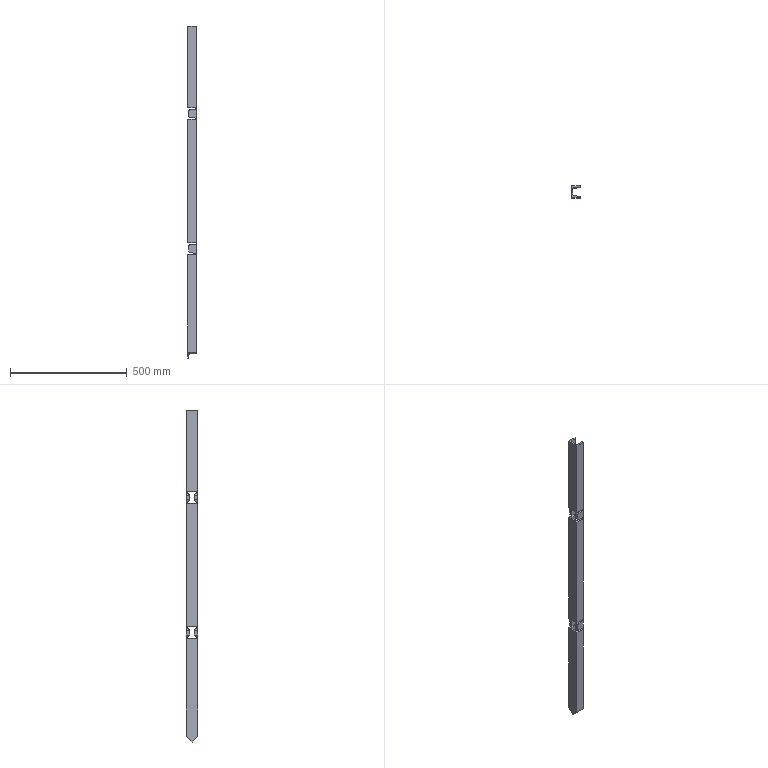Part | STEP file | DIN 1026-1 U 50 1785357074696 | 7 solids | 91 faces | box 38 x 50 x 1422 mm | volume 960658 mm3 | plane 55 | cylinder 36 | commonest cylinder face diameters 7 x18 14 x18